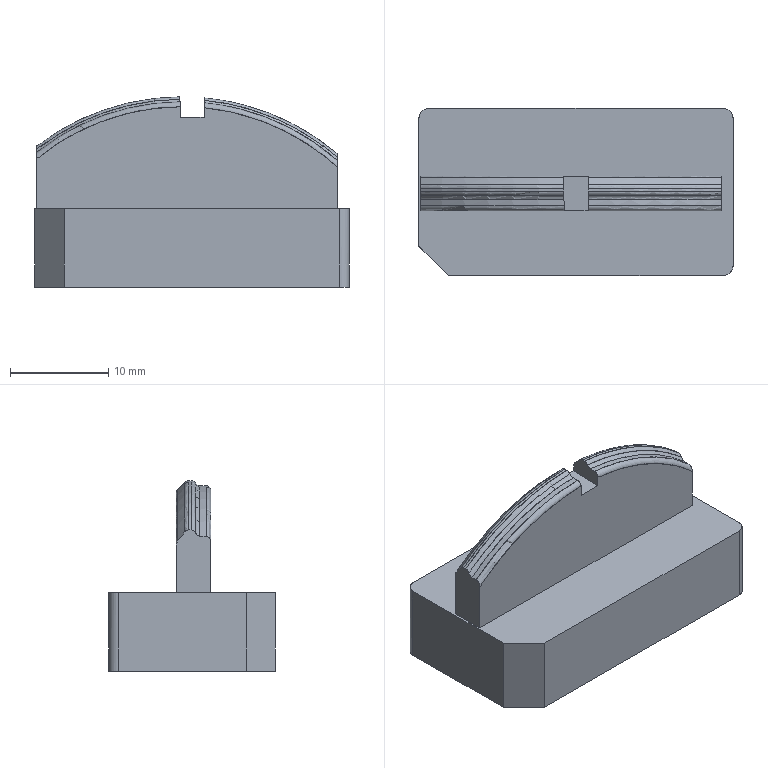NC program | PowerMill | posted with a generic post | part box 32 x 17 x 19.383 mm
Lines 8610 to 9354 of 94163:
N8707 M6
N8708 S22000 M03
N8709 G00 G90 X0.0 Y0.0
N8710 G43 Z10.803 H22
N8711
N8712 G05 P10000 R8
N8713 X15.4268 Y-3.0703
N8714 Z-6.8835
N8715 G01 Z-8.0835 F1200.0
N8716 X15.4156 Y-3.0814 Z-8.097 F2000.0
N8717 X15.3964 Y-3.1007 Z-8.1231
N8718 X15.376 Y-3.121 Z-8.1542
N8719 X15.3523 Y-3.1447 Z-8.1945
N8720 X15.3274 Y-3.1696 Z-8.242
N8721 X15.3089 Y-3.1881 Z-8.2813
N8722 X15.295 Y-3.2021 Z-8.3142
N8723 X15.2826 Y-3.2144 Z-8.3478
N8724 X15.2414 Y-3.2443 Z-8.4199
N8725 X15.199 Y-3.2705 Z-8.4928
N8726 X15.1554 Y-3.2929 Z-8.5663
N8727 X15.1411 Y-3.2994 Z-8.5902
N8728 X15.1525 Y-3.288 Z-8.5245
N8729 X15.1666 Y-3.2739 Z-8.4598
N8730 X15.1833 Y-3.2571 Z-8.3965
N8731 X15.2025 Y-3.2379 Z-8.3352
N8732 X15.224 Y-3.2164 Z-8.2762
N8733 X15.2477 Y-3.1928 Z-8.22
N8734 X15.2732 Y-3.1672 Z-8.1668
N8735 X15.3005 Y-3.14 Z-8.117
N8736 X15.3293 Y-3.1111 Z-8.0706
N8737 X15.3595 Y-3.0809 Z-8.0279
N8738 X15.3909 Y-3.0495 Z-7.989
N8739 X15.4234 Y-3.0171 Z-7.9539
N8740 X15.4567 Y-2.9837 Z-7.9227
N8741 X15.4909 Y-2.9496 Z-7.8955
N8742 X15.5257 Y-2.9148 Z-7.8721
N8743 X15.546 Y-2.8945 Z-7.8605
N8744 X15.61 Y-2.7738 Z-7.744
N8745 X15.5875 Y-2.7964 Z-7.7488
N8746 X15.572 Y-2.8119 Z-7.7542
N8747 X15.5342 Y-2.8497 Z-7.7703
N8748 X15.4967 Y-2.8871 Z-7.7904
N8749 X15.4598 Y-2.9241 Z-7.8144
N8750 X15.4234 Y-2.9604 Z-7.8424
N8751 X15.3878 Y-2.996 Z-7.8743
N8752 X15.3531 Y-3.0307 Z-7.9101
N8753 X15.3195 Y-3.0644 Z-7.9497
N8754 X15.2879 Y-3.0959 Z-7.9919
N8755 X15.2579 Y-3.126 Z-8.0376
N8756 X15.2291 Y-3.1548 Z-8.087
N8757 X15.2018 Y-3.1821 Z-8.1402
N8758 X15.1762 Y-3.2077 Z-8.1968
N8759 X15.1525 Y-3.2314 Z-8.2566
N8760 X15.1309 Y-3.253 Z-8.3191
N8761 X15.1116 Y-3.2723 Z-8.3838
N8762 X15.095 Y-3.2889 Z-8.45
N8763 X15.0811 Y-3.3028 Z-8.5166
N8764 X15.0702 Y-3.3137 Z-8.5828
N8765 X15.0621 Y-3.3217 Z-8.6478
N8766 X14.9924 Y-3.3349 Z-8.675
N8767 X14.9992 Y-3.3281 Z-8.608
N8768 X15.0089 Y-3.3184 Z-8.5397
N8769 X15.0217 Y-3.3056 Z-8.4697
N8770 X15.0377 Y-3.2896 Z-8.3981
N8771 X15.0557 Y-3.2716 Z-8.3289
N8772 X15.0757 Y-3.2516 Z-8.2631
N8773 X15.0976 Y-3.2297 Z-8.2007
N8774 X15.1214 Y-3.2059 Z-8.1417
N8775 X15.147 Y-3.1803 Z-8.0858
N8776 X15.1745 Y-3.1528 Z-8.0331
N8777 X15.2038 Y-3.1235 Z-7.9835
N8778 X15.2349 Y-3.0924 Z-7.9367
N8779 X15.2665 Y-3.0608 Z-7.8947
N8780 X15.299 Y-3.0284 Z-7.8564
N8781 X15.3344 Y-2.9929 Z-7.8197
N8782 X15.3723 Y-2.955 Z-7.7852
N8783 X15.4115 Y-2.9158 Z-7.7544
N8784 X15.4509 Y-2.8764 Z-7.7277
N8785 X15.49 Y-2.8373 Z-7.7054
N8786 X15.5282 Y-2.7991 Z-7.6877
N8787 X15.5652 Y-2.7621 Z-7.6743
N8788 X15.6008 Y-2.7266 Z-7.6652
N8789 X15.6348 Y-2.6925 Z-7.6601
N8790 X15.6524 Y-2.6749 Z-7.659
N8791 X15.6845 Y-2.5863 Z-7.5915
N8792 X15.6827 Y-2.588 Z-7.5913
N8793 X15.6486 Y-2.6222 Z-7.59
N8794 X15.6126 Y-2.6582 Z-7.5924
N8795 X15.5749 Y-2.6959 Z-7.5989
N8796 X15.5355 Y-2.7352 Z-7.6094
N8797 X15.4947 Y-2.776 Z-7.6242
N8798 X15.4528 Y-2.818 Z-7.6435
N8799 X15.4102 Y-2.8606 Z-7.6672
N8800 X15.3676 Y-2.9031 Z-7.6951
N8801 X15.326 Y-2.9447 Z-7.7268
N8802 X15.2868 Y-2.984 Z-7.761
N8803 X15.2505 Y-3.0202 Z-7.7969
N8804 X15.2176 Y-3.0532 Z-7.8339
N8805 X15.1882 Y-3.0826 Z-7.8714
N8806 X15.1612 Y-3.1095 Z-7.9101
N8807 X15.1314 Y-3.1394 Z-7.9582
N8808 X15.1032 Y-3.1676 Z-8.0097
N8809 X15.0766 Y-3.1941 Z-8.0646
N8810 X15.0517 Y-3.219 Z-8.123
N8811 X15.0287 Y-3.242 Z-8.1847
N8812 X15.0076 Y-3.2632 Z-8.2499
N8813 X14.9884 Y-3.2823 Z-8.3183
N8814 X14.9714 Y-3.2994 Z-8.3899
N8815 X14.9566 Y-3.3141 Z-8.4643
N8816 X14.9442 Y-3.3265 Z-8.5414
N8817 X14.9343 Y-3.3364 Z-8.6204
N8818 X14.927 Y-3.3437 Z-8.7008
N8819 X14.8662 Y-3.348 Z-8.6975
N8820 X14.8731 Y-3.341 Z-8.6103
N8821 X14.8824 Y-3.3317 Z-8.527
N8822 X14.894 Y-3.3201 Z-8.4474
N8823 X14.9079 Y-3.3063 Z-8.3713
N8824 X14.9239 Y-3.2903 Z-8.2984
N8825 X14.9417 Y-3.2725 Z-8.2303
N8826 X14.9615 Y-3.2526 Z-8.1649
N8827 X14.9835 Y-3.2307 Z-8.1026
N8828 X15.0074 Y-3.2068 Z-8.0433
N8829 X15.0333 Y-3.1809 Z-7.987
N8830 X15.0611 Y-3.1531 Z-7.9337
N8831 X15.0908 Y-3.1234 Z-7.8834
N8832 X15.1224 Y-3.0918 Z-7.836
N8833 X15.1558 Y-3.0584 Z-7.7916
N8834 X15.189 Y-3.0251 Z-7.7526
N8835 X15.2246 Y-2.9896 Z-7.716
N8836 X15.2625 Y-2.9517 Z-7.6819
N8837 X15.3026 Y-2.9116 Z-7.6506
N8838 X15.3448 Y-2.8694 Z-7.622
N8839 X15.3732 Y-2.841 Z-7.6052
N8840 X15.4021 Y-2.8121 Z-7.5901
N8841 X15.4316 Y-2.7826 Z-7.5765
N8842 X15.466 Y-2.7482 Z-7.5628
N8843 X15.506 Y-2.7082 Z-7.5494
N8844 X15.5505 Y-2.6637 Z-7.5379
N8845 X15.5927 Y-2.6215 Z-7.5306
N8846 X15.6313 Y-2.5828 Z-7.5274
N8847 X15.6664 Y-2.5478 Z-7.5279
N8848 X15.6982 Y-2.516 Z-7.5318
N8849 X15.7135 Y-2.5007 Z-7.535
N8850 X15.7387 Y-2.4189 Z-7.4879
N8851 X15.7303 Y-2.4273 Z-7.4851
N8852 X15.7013 Y-2.4563 Z-7.4777
N8853 X15.6691 Y-2.4885 Z-7.4728
N8854 X15.6332 Y-2.5244 Z-7.4708
N8855 X15.5932 Y-2.5644 Z-7.472
N8856 X15.5488 Y-2.6088 Z-7.4769
N8857 X15.5002 Y-2.6574 Z-7.486
N8858 X15.4505 Y-2.7071 Z-7.499
N8859 X15.406 Y-2.7516 Z-7.514
N8860 X15.3672 Y-2.7904 Z-7.5297
N8861 X15.3336 Y-2.824 Z-7.5457
N8862 X15.3047 Y-2.8529 Z-7.5615
N8863 X15.2705 Y-2.8871 Z-7.5831
N8864 X15.2299 Y-2.9277 Z-7.6124
N8865 X15.1908 Y-2.9668 Z-7.645
N8866 X15.1534 Y-3.0042 Z-7.6808
N8867 X15.1176 Y-3.04 Z-7.7197
N8868 X15.0835 Y-3.0741 Z-7.7618
N8869 X15.0511 Y-3.1065 Z-7.807
N8870 X15.0205 Y-3.1371 Z-7.8554
N8871 X14.9917 Y-3.1659 Z-7.9068
N8872 X14.9648 Y-3.1928 Z-7.9613
N8873 X14.9399 Y-3.2177 Z-8.0189
N8874 X14.9169 Y-3.2407 Z-8.0794
N8875 X14.8959 Y-3.2617 Z-8.1429
N8876 X14.877 Y-3.2806 Z-8.2092
N8877 X14.86 Y-3.2976 Z-8.2794
N8878 X14.845 Y-3.3126 Z-8.3533
N8879 X14.8321 Y-3.3255 Z-8.431
N8880 X14.8215 Y-3.3361 Z-8.5126
N8881 X14.8132 Y-3.3444 Z-8.598
N8882 X14.8073 Y-3.3503 Z-8.687
N8883 X14.7489 Y-3.3521 Z-8.6765
N8884 X14.7535 Y-3.3475 Z-8.5876
N8885 X14.7607 Y-3.3404 Z-8.5016
N8886 X14.7702 Y-3.3308 Z-8.4187
N8887 X14.7821 Y-3.3189 Z-8.3393
N8888 X14.7963 Y-3.3047 Z-8.2633
N8889 X14.8126 Y-3.2885 Z-8.1908
N8890 X14.8309 Y-3.2701 Z-8.1219
N8891 X14.8512 Y-3.2498 Z-8.0563
N8892 X14.8734 Y-3.2276 Z-7.9942
N8893 X14.8975 Y-3.2036 Z-7.9354
N8894 X14.9233 Y-3.1777 Z-7.88
N8895 X14.951 Y-3.1501 Z-7.8278
N8896 X14.9803 Y-3.1207 Z-7.7788
N8897 X15.0113 Y-3.0897 Z-7.7329
N8898 X15.044 Y-3.057 Z-7.6902
N8899 X15.0787 Y-3.0223 Z-7.6502
N8900 X15.1155 Y-2.9856 Z-7.6128
N8901 X15.154 Y-2.947 Z-7.5786
N8902 X15.1944 Y-2.9067 Z-7.5474
N8903 X15.2364 Y-2.8646 Z-7.5194
N8904 X15.2801 Y-2.8209 Z-7.4947
N8905 X15.3253 Y-2.7757 Z-7.4735
N8906 X15.3718 Y-2.7292 Z-7.4558
N8907 X15.4196 Y-2.6815 Z-7.4418
N8908 X15.4683 Y-2.6327 Z-7.4314
N8909 X15.5236 Y-2.5775 Z-7.4229
N8910 X15.5727 Y-2.5284 Z-7.4186
N8911 X15.6175 Y-2.4836 Z-7.4182
N8912 X15.659 Y-2.4421 Z-7.4214
N8913 X15.6978 Y-2.4032 Z-7.428
N8914 X15.7345 Y-2.3666 Z-7.4379
N8915 X15.7593 Y-2.3418 Z-7.447
N8916 X15.7805 Y-2.264 Z-7.4113
N8917 X15.7689 Y-2.2756 Z-7.4063
N8918 X15.7299 Y-2.3145 Z-7.3921
N8919 X15.6887 Y-2.3558 Z-7.3811
N8920 X15.645 Y-2.3995 Z-7.3733
N8921 X15.5982 Y-2.4462 Z-7.3689
N8922 X15.5478 Y-2.4967 Z-7.3681
N8923 X15.4927 Y-2.5518 Z-7.3709
N8924 X15.4411 Y-2.6034 Z-7.3765
N8925 X15.3906 Y-2.6538 Z-7.3853
N8926 X15.3415 Y-2.703 Z-7.3978
N8927 X15.2937 Y-2.7507 Z-7.4139
N8928 X15.2476 Y-2.7969 Z-7.4334
N8929 X15.203 Y-2.8414 Z-7.4564
N8930 X15.1603 Y-2.8842 Z-7.4826
N8931 X15.1193 Y-2.9251 Z-7.5119
N8932 X15.0802 Y-2.9642 Z-7.5443
N8933 X15.0429 Y-3.0016 Z-7.5797
N8934 X15.0073 Y-3.0371 Z-7.618
N8935 X14.9735 Y-3.071 Z-7.6592
N8936 X14.9413 Y-3.1032 Z-7.7034
N8937 X14.9109 Y-3.1336 Z-7.7507
N8938 X14.8822 Y-3.1623 Z-7.801
N8939 X14.8552 Y-3.1892 Z-7.8545
N8940 X14.8301 Y-3.2143 Z-7.9111
N8941 X14.8069 Y-3.2376 Z-7.971
N8942 X14.7855 Y-3.259 Z-8.0342
N8943 X14.7661 Y-3.2784 Z-8.1008
N8944 X14.7487 Y-3.2958 Z-8.1708
N8945 X14.7334 Y-3.3111 Z-8.2444
N8946 X14.7203 Y-3.3242 Z-8.3214
N8947 X14.7094 Y-3.3351 Z-8.402
N8948 X14.7008 Y-3.3436 Z-8.4862
N8949 X14.6947 Y-3.3497 Z-8.5738
N8950 X14.6912 Y-3.3533 Z-8.6645
N8951 X14.6337 Y-3.3542 Z-8.6512
N8952 X14.6363 Y-3.3516 Z-8.5591
N8953 X14.6415 Y-3.3464 Z-8.4701
N8954 X14.6492 Y-3.3387 Z-8.3845
N8955 X14.6593 Y-3.3286 Z-8.3024
N8956 X14.6716 Y-3.3163 Z-8.2238
N8957 X14.6862 Y-3.3017 Z-8.1488
N8958 X14.7028 Y-3.2851 Z-8.0774
N8959 X14.7215 Y-3.2664 Z-8.0094
N8960 X14.7422 Y-3.2457 Z-7.9448
N8961 X14.7648 Y-3.2231 Z-7.8836
N8962 X14.7892 Y-3.1987 Z-7.8257
N8963 X14.8155 Y-3.1724 Z-7.771
N8964 X14.8435 Y-3.1444 Z-7.7196
N8965 X14.8733 Y-3.1146 Z-7.6712
N8966 X14.9048 Y-3.0831 Z-7.626
N8967 X14.938 Y-3.0499 Z-7.5838
N8968 X14.9728 Y-3.0151 Z-7.5446
N8969 X15.0092 Y-2.9787 Z-7.5085
N8970 X15.0469 Y-2.941 Z-7.4755
N8971 X15.0864 Y-2.9015 Z-7.4454
N8972 X15.1278 Y-2.8601 Z-7.4183
N8973 X15.1714 Y-2.8165 Z-7.3941
N8974 X15.2175 Y-2.7704 Z-7.3727
N8975 X15.2661 Y-2.7218 Z-7.3542
N8976 X15.2963 Y-2.6916 Z-7.3445
N8977 X15.3272 Y-2.6607 Z-7.3366
N8978 X15.3628 Y-2.6251 Z-7.3297
N8979 X15.4038 Y-2.5841 Z-7.324
N8980 X15.451 Y-2.5369 Z-7.32
N8981 X15.5051 Y-2.4828 Z-7.3186
N8982 X15.5629 Y-2.425 Z-7.3207
N8983 X15.6147 Y-2.3732 Z-7.326
N8984 X15.6602 Y-2.3277 Z-7.3336
N8985 X15.7 Y-2.2879 Z-7.343
N8986 X15.7349 Y-2.253 Z-7.3539
N8987 X15.7656 Y-2.2223 Z-7.3661
N8988 X15.7946 Y-2.1933 Z-7.3808
N8989 X15.797 Y-2.1909 Z-7.3822
N8990 X15.8099 Y-2.1214 Z-7.3564
N8991 X15.7858 Y-2.1455 Z-7.3418
N8992 X15.7525 Y-2.1789 Z-7.3253
N8993 X15.7148 Y-2.2166 Z-7.3105
N8994 X15.6718 Y-2.2595 Z-7.2976
N8995 X15.6227 Y-2.3086 Z-7.2866
N8996 X15.568 Y-2.3634 Z-7.2778
N8997 X15.5206 Y-2.4108 Z-7.2724
N8998 X15.4638 Y-2.4675 Z-7.2688
N8999 X15.4086 Y-2.5228 Z-7.2692
N9000 X15.3547 Y-2.5766 Z-7.2734
N9001 X15.3023 Y-2.629 Z-7.2814
N9002 X15.2513 Y-2.68 Z-7.2931
N9003 X15.2017 Y-2.7297 Z-7.3084
N9004 X15.1534 Y-2.778 Z-7.3273
N9005 X15.1095 Y-2.8218 Z-7.348
N9006 X15.0666 Y-2.8647 Z-7.3723
N9007 X15.0249 Y-2.9064 Z-7.4001
N9008 X14.9846 Y-2.9467 Z-7.4315
N9009 X14.9458 Y-2.9855 Z-7.4662
N9010 X14.9087 Y-3.0227 Z-7.5042
N9011 X14.8732 Y-3.0581 Z-7.5453
N9012 X14.8396 Y-3.0917 Z-7.5895
N9013 X14.8079 Y-3.1234 Z-7.6365
N9014 X14.7783 Y-3.153 Z-7.6863
N9015 X14.7507 Y-3.1806 Z-7.7388
N9016 X14.725 Y-3.2063 Z-7.7942
N9017 X14.7012 Y-3.2301 Z-7.8529
N9018 X14.6793 Y-3.2521 Z-7.9147
N9019 X14.6592 Y-3.2721 Z-7.98
N9020 X14.6412 Y-3.2901 Z-8.0487
N9021 X14.6252 Y-3.3061 Z-8.121
N9022 X14.6113 Y-3.32 Z-8.1969
N9023 X14.5995 Y-3.3318 Z-8.2766
N9024 X14.5901 Y-3.3412 Z-8.3602
N9025 X14.5831 Y-3.3482 Z-8.4467
N9026 X14.5786 Y-3.3527 Z-8.5365
N9027 X14.5768 Y-3.3545 Z-8.6297
N9028 Z-8.638
N9029 X14.5202 Y-3.3546 Z-8.6211
N9030 Z-8.5883
N9031 X14.5218 Y-3.3529 Z-8.4943
N9032 X14.5261 Y-3.3487 Z-8.4039
N9033 X14.5329 Y-3.3419 Z-8.317
N9034 X14.542 Y-3.3327 Z-8.2339
N9035 X14.5535 Y-3.3213 Z-8.1544
N9036 X14.5672 Y-3.3076 Z-8.0786
N9037 X14.583 Y-3.2917 Z-8.0062
N9038 X14.6009 Y-3.2738 Z-7.9373
N9039 X14.6209 Y-3.2539 Z-7.8717
N9040 X14.6428 Y-3.232 Z-7.8094
N9041 X14.6666 Y-3.2082 Z-7.7503
N9042 X14.6923 Y-3.1825 Z-7.6943
N9043 X14.7198 Y-3.1549 Z-7.6415
N9044 X14.7492 Y-3.1256 Z-7.5917
N9045 X14.7803 Y-3.0944 Z-7.5449
N9046 X14.8132 Y-3.0615 Z-7.501
N9047 X14.8477 Y-3.027 Z-7.4603
N9048 X14.8838 Y-2.9909 Z-7.4228
N9049 X14.9216 Y-2.9531 Z-7.3885
N9050 X14.9613 Y-2.9134 Z-7.357
N9051 X15.003 Y-2.8717 Z-7.3286
N9052 X15.0467 Y-2.8281 Z-7.3031
N9053 X15.0923 Y-2.7825 Z-7.2809
N9054 X15.1399 Y-2.7348 Z-7.2618
N9055 X15.1895 Y-2.6853 Z-7.246
N9056 X15.2411 Y-2.6337 Z-7.2337
N9057 X15.2946 Y-2.5802 Z-7.2248
N9058 X15.35 Y-2.5248 Z-7.2197
N9059 X15.3784 Y-2.4963 Z-7.2186
N9060 X15.4073 Y-2.4675 Z-7.2188
N9061 X15.441 Y-2.4337 Z-7.2205
N9062 X15.4806 Y-2.3941 Z-7.2241
N9063 X15.5278 Y-2.3469 Z-7.2304
N9064 X15.5849 Y-2.2899 Z-7.2408
N9065 X15.6404 Y-2.2344 Z-7.254
N9066 X15.6863 Y-2.1885 Z-7.2678
N9067 X15.725 Y-2.1498 Z-7.2817
N9068 X15.7579 Y-2.1168 Z-7.296
N9069 X15.7861 Y-2.0887 Z-7.3104
N9070 X15.812 Y-2.0628 Z-7.3264
N9071 X15.8212 Y-2.0536 Z-7.3329
N9072 X15.8305 Y-1.9877 Z-7.3116
N9073 X15.8244 Y-1.9938 Z-7.307
N9074 X15.7966 Y-2.0216 Z-7.2886
N9075 X15.7675 Y-2.0507 Z-7.2722
N9076 X15.7335 Y-2.0847 Z-7.2558
N9077 X15.6936 Y-2.1246 Z-7.2392
N9078 X15.6464 Y-2.1718 Z-7.2226
N9079 X15.5896 Y-2.2286 Z-7.2058
N9080 X15.5304 Y-2.2878 Z-7.1917
N9081 X15.4811 Y-2.3371 Z-7.1824
N9082 X15.4395 Y-2.3787 Z-7.1763
N9083 X15.4039 Y-2.4143 Z-7.1725
N9084 X15.3731 Y-2.4451 Z-7.1704
N9085 X15.3423 Y-2.4759 Z-7.1698
N9086 X15.2844 Y-2.5338 Z-7.1718
N9087 X15.2294 Y-2.5888 Z-7.1773
N9088 X15.1769 Y-2.6413 Z-7.1864
N9089 X15.1266 Y-2.6915 Z-7.1988
N9090 X15.0785 Y-2.7397 Z-7.2146
N9091 X15.0322 Y-2.786 Z-7.2337
N9092 X14.9876 Y-2.8306 Z-7.2562
N9093 X14.9446 Y-2.8736 Z-7.2819
N9094 X14.9031 Y-2.9151 Z-7.3108
N9095 X14.8638 Y-2.9544 Z-7.3423
N9096 X14.826 Y-2.9922 Z-7.3768
N9097 X14.7899 Y-3.0283 Z-7.4142
N9098 X14.7555 Y-3.0627 Z-7.4546
N9099 X14.7228 Y-3.0954 Z-7.498
N9100 X14.6918 Y-3.1264 Z-7.5445
N9101 X14.6626 Y-3.1556 Z-7.594
N9102 X14.6352 Y-3.183 Z-7.6467
N9103 X14.6096 Y-3.2086 Z-7.7025
N9104 X14.5858 Y-3.2324 Z-7.7616
N9105 X14.564 Y-3.2542 Z-7.8239
N9106 X14.5441 Y-3.274 Z-7.8895
N9107 X14.5263 Y-3.2919 Z-7.9586
N9108 X14.5105 Y-3.3077 Z-8.031
N9109 X14.4968 Y-3.3214 Z-8.107
N9110 X14.4853 Y-3.3329 Z-8.1866
N9111 X14.4762 Y-3.342 Z-8.2693
N9112 X14.4695 Y-3.3487 Z-8.3555
N9113 X14.4653 Y-3.3529 Z-8.4455
N9114 X14.4636 Y-3.3546 Z-8.5398
N9115 Z-8.5922
N9116 X14.407 Z-8.5633
N9117 Z-8.4931
N9118 X14.4085 Y-3.3531 Z-8.4005
N9119 X14.4126 Y-3.349 Z-8.3114
N9120 X14.4193 Y-3.3423 Z-8.2247
N9121 X14.4285 Y-3.3332 Z-8.1406
N9122 X14.4397 Y-3.3219 Z-8.0612
N9123 X14.4531 Y-3.3085 Z-7.9858
N9124 X14.4686 Y-3.293 Z-7.9142
N9125 X14.4862 Y-3.2755 Z-7.846
N9126 X14.5058 Y-3.2558 Z-7.781
N9127 X14.5275 Y-3.2341 Z-7.719
N9128 X14.5512 Y-3.2104 Z-7.6598
N9129 X14.577 Y-3.1847 Z-7.6034
N9130 X14.6049 Y-3.1567 Z-7.5492
N9131 X14.634 Y-3.1277 Z-7.4993
N9132 X14.665 Y-3.0966 Z-7.4521
N9133 X14.698 Y-3.0636 Z-7.4079
N9134 X14.7329 Y-3.0288 Z-7.3666
N9135 X14.7696 Y-2.9921 Z-7.3283
N9136 X14.808 Y-2.9536 Z-7.2932
N9137 X14.8481 Y-2.9135 Z-7.2612
N9138 X14.8899 Y-2.8717 Z-7.2326
N9139 X14.9329 Y-2.8287 Z-7.2075
N9140 X14.9796 Y-2.782 Z-7.1845
N9141 X15.0272 Y-2.7344 Z-7.1651
N9142 X15.0763 Y-2.6854 Z-7.1492
N9143 X15.1269 Y-2.6348 Z-7.1368
N9144 X15.1793 Y-2.5823 Z-7.128
N9145 X15.2337 Y-2.5279 Z-7.1228
N9146 X15.2905 Y-2.4711 Z-7.1212
N9147 X15.343 Y-2.4186 Z-7.123
N9148 X15.377 Y-2.3846 Z-7.126
N9149 X15.4115 Y-2.3501 Z-7.1306
N9150 X15.4514 Y-2.3103 Z-7.1376
N9151 X15.4979 Y-2.2637 Z-7.1476
N9152 X15.5531 Y-2.2085 Z-7.1619
N9153 X15.6176 Y-2.1441 Z-7.182
N9154 X15.6719 Y-2.0897 Z-7.2022
N9155 X15.7176 Y-2.0441 Z-7.2217
N9156 X15.7564 Y-2.0052 Z-7.2408
N9157 X15.7897 Y-1.9719 Z-7.2595
N9158 X15.8206 Y-1.9411 Z-7.2794
N9159 X15.8389 Y-1.9228 Z-7.2929
N9160 X15.8444 Y-1.8606 Z-7.2786
N9161 X15.8234 Y-1.8817 Z-7.2611
N9162 X15.7936 Y-1.9115 Z-7.2398
N9163 X15.7582 Y-1.9469 Z-7.2182
N9164 X15.7154 Y-1.9897 Z-7.1958
N9165 X15.6628 Y-2.0423 Z-7.1721
N9166 X15.6171 Y-2.0879 Z-7.1538
N9167 X15.5801 Y-2.1249 Z-7.14
N9168 X15.5453 Y-2.1597 Z-7.1277
N9169 X15.482 Y-2.2231 Z-7.1084
N9170 X15.4203 Y-2.2848 Z-7.0934
N9171 X15.3599 Y-2.3451 Z-7.0826
N9172 X15.3008 Y-2.4042 Z-7.0759
N9173 X15.2428 Y-2.4623 Z-7.0732
N9174 X15.185 Y-2.52 Z-7.0744
N9175 X15.1297 Y-2.5754 Z-7.0794
N9176 X15.0762 Y-2.6288 Z-7.0879
N9177 X15.0248 Y-2.6802 Z-7.0999
N9178 X14.9754 Y-2.7296 Z-7.1153
N9179 X14.928 Y-2.7771 Z-7.1341
N9180 X14.8824 Y-2.8227 Z-7.1561
N9181 X14.8386 Y-2.8664 Z-7.1814
N9182 X14.7967 Y-2.9084 Z-7.2098
N9183 X14.7565 Y-2.9485 Z-7.2413
N9184 X14.7181 Y-2.9869 Z-7.2759
N9185 X14.6815 Y-3.0236 Z-7.3135
N9186 X14.6465 Y-3.0585 Z-7.3541
N9187 X14.6136 Y-3.0915 Z-7.3974
N9188 X14.5822 Y-3.1229 Z-7.4438
N9189 X14.5528 Y-3.1523 Z-7.4929
N9190 X14.5252 Y-3.1799 Z-7.5452
N9191 X14.4993 Y-3.2057 Z-7.6007
N9192 X14.4753 Y-3.2297 Z-7.6593
N9193 X14.4532 Y-3.2518 Z-7.7213
N9194 X14.4331 Y-3.272 Z-7.7865
N9195 X14.4149 Y-3.2902 Z-7.8552
N9196 X14.3988 Y-3.3063 Z-7.9273
N9197 X14.3848 Y-3.3202 Z-8.0028
N9198 X14.3731 Y-3.3319 Z-8.0818
N9199 X14.3637 Y-3.3413 Z-8.1643
N9200 X14.3568 Y-3.3483 Z-8.25
N9201 X14.3524 Y-3.3527 Z-8.3387
N9202 X14.3505 Y-3.3545 Z-8.4322
N9203 Z-8.5344
N9204 X14.2939 Y-3.3546 Z-8.489
N9205 Z-8.3864
N9206 X14.2956 Y-3.3529 Z-8.2949
N9207 X14.3 Y-3.3485 Z-8.2059
N9208 X14.3069 Y-3.3415 Z-8.1195
N9209 X14.3165 Y-3.332 Z-8.0356
N9210 X14.327 Y-3.3215 Z-7.9629
N9211 X14.3405 Y-3.308 Z-7.8881
N9212 X14.3562 Y-3.2923 Z-7.8164
N9213 X14.374 Y-3.2744 Z-7.7476
N9214 X14.394 Y-3.2545 Z-7.682
N9215 X14.416 Y-3.2325 Z-7.6195
N9216 X14.44 Y-3.2085 Z-7.5601
N9217 X14.4658 Y-3.1826 Z-7.5039
N9218 X14.4936 Y-3.1549 Z-7.4508
N9219 X14.5231 Y-3.1254 Z-7.4008
N9220 X14.5543 Y-3.0942 Z-7.3539
N9221 X14.5873 Y-3.0612 Z-7.3102
N9222 X14.6219 Y-3.0266 Z-7.2695
N9223 X14.6582 Y-2.9903 Z-7.232
N9224 X14.6962 Y-2.9523 Z-7.1974
N9225 X14.7366 Y-2.9119 Z-7.1653
N9226 X14.7788 Y-2.8697 Z-7.1363
N9227 X14.8228 Y-2.8257 Z-7.1105
N9228 X14.8685 Y-2.78 Z-7.088
N9229 X14.9158 Y-2.7327 Z-7.0689
N9230 X14.9645 Y-2.684 Z-7.0534
N9231 X15.0141 Y-2.6344 Z-7.0414
N9232 X15.0675 Y-2.581 Z-7.0322
N9233 X15.122 Y-2.5265 Z-7.0267
N9234 X15.178 Y-2.4705 Z-7.0249
N9235 X15.2358 Y-2.4127 Z-7.027
N9236 X15.2957 Y-2.3527 Z-7.0332
N9237 X15.3582 Y-2.2903 Z-7.0434
N9238 X15.3876 Y-2.2609 Z-7.0494
N9239 X15.4158 Y-2.2327 Z-7.0562
N9240 X15.4442 Y-2.2043 Z-7.0641
N9241 X15.4774 Y-2.1711 Z-7.0744
N9242 X15.5167 Y-2.1318 Z-7.0878
N9243 X15.5642 Y-2.0843 Z-7.1056
N9244 X15.6245 Y-2.024 Z-7.1306
N9245 X15.6799 Y-1.9686 Z-7.1564
N9246 X15.7238 Y-1.9247 Z-7.1791
N9247 X15.76 Y-1.8885 Z-7.1998
N9248 X15.7905 Y-1.858 Z-7.2191
N9249 X15.8162 Y-1.8323 Z-7.2373
N9250 X15.8408 Y-1.8077 Z-7.2572
N9251 X15.8491 Y-1.7994 Z-7.2648
N9252 X15.855 Y-1.737 Z-7.2543
N9253 X15.8285 Y-1.7634 Z-7.2313
N9254 X15.7978 Y-1.7942 Z-7.2078
N9255 X15.7642 Y-1.8277 Z-7.1848
N9256 X15.7251 Y-1.8668 Z-7.1606
N9257 X15.6791 Y-1.9128 Z-7.1348
N9258 X15.6241 Y-1.9678 Z-7.1069
N9259 X15.5572 Y-2.0348 Z-7.0766
N9260 X15.4966 Y-2.0953 Z-7.0522
N9261 X15.446 Y-2.146 Z-7.034
N9262 X15.4026 Y-2.1893 Z-7.02
N9263 X15.3651 Y-2.2269 Z-7.0092
N9264 X15.3304 Y-2.2615 Z-7.0007
N9265 X15.2956 Y-2.2964 Z-6.9937
N9266 X15.2388 Y-2.3532 Z-6.985
N9267 X15.1802 Y-2.4117 Z-6.9791
N9268 X15.123 Y-2.4689 Z-6.9769
N9269 X15.069 Y-2.5229 Z-6.9785
N9270 X15.0168 Y-2.5751 Z-6.9836
N9271 X14.9647 Y-2.6272 Z-6.9921
N9272 X14.9164 Y-2.6755 Z-7.0034
N9273 X14.8669 Y-2.725 Z-7.0188
N9274 X14.8191 Y-2.7729 Z-7.0376
N9275 X14.7729 Y-2.819 Z-7.0598
N9276 X14.7286 Y-2.8633 Z-7.0853
N9277 X14.6862 Y-2.9057 Z-7.1138
N9278 X14.6457 Y-2.9462 Z-7.1454
N9279 X14.6072 Y-2.9848 Z-7.1799
N9280 X14.5705 Y-3.0214 Z-7.2173
N9281 X14.5355 Y-3.0564 Z-7.2577
N9282 X14.5023 Y-3.0896 Z-7.301
N9283 X14.4708 Y-3.1211 Z-7.3472
N9284 X14.4412 Y-3.1508 Z-7.3965
N9285 X14.4133 Y-3.1786 Z-7.4487
N9286 X14.3873 Y-3.2047 Z-7.504
N9287 X14.3631 Y-3.2288 Z-7.5625
N9288 X14.3409 Y-3.251 Z-7.6241
N9289 X14.3207 Y-3.2713 Z-7.689
N9290 X14.3024 Y-3.2895 Z-7.7572
N9291 X14.2863 Y-3.3056 Z-7.8287
N9292 X14.2723 Y-3.3196 Z-7.9037
N9293 X14.2605 Y-3.3314 Z-7.9822
N9294 X14.251 Y-3.3409 Z-8.0643
N9295 X14.2439 Y-3.348 Z-8.1499
N9296 X14.2393 Y-3.3526 Z-8.239
N9297 X14.2374 Y-3.3545 Z-8.3316
N9298 Z-8.4414
N9299 X14.1808 Z-8.3939
N9300 Z-8.2834
N9301 X14.1828 Y-3.3525 Z-8.1903
N9302 X14.1875 Y-3.3479 Z-8.101
N9303 X14.1945 Y-3.3408 Z-8.0157
N9304 X14.204 Y-3.3314 Z-7.934
N9305 X14.2157 Y-3.3196 Z-7.8559
N9306 X14.2297 Y-3.3056 Z-7.7814
N9307 X14.2459 Y-3.2895 Z-7.7102
N9308 X14.2641 Y-3.2713 Z-7.6423
N9309 X14.2844 Y-3.251 Z-7.5775
N9310 X14.3067 Y-3.2286 Z-7.5158
N9311 X14.331 Y-3.2043 Z-7.4571
N9312 X14.3573 Y-3.1781 Z-7.4013
N9313 X14.3849 Y-3.1504 Z-7.3494
N9314 X14.4146 Y-3.1208 Z-7.3
N9315 X14.4462 Y-3.0891 Z-7.2535
N9316 X14.4798 Y-3.0556 Z-7.2098
N9317 X14.5152 Y-3.0202 Z-7.169
N9318 X14.5525 Y-2.9829 Z-7.1313
N9319 X14.5916 Y-2.9437 Z-7.0965
N9320 X14.6325 Y-2.9028 Z-7.0649
N9321 X14.6751 Y-2.8602 Z-7.0366
N9322 X14.7194 Y-2.8159 Z-7.0114
N9323 X14.7654 Y-2.77 Z-6.9897
N9324 X14.8125 Y-2.7228 Z-6.9713
N9325 X14.8631 Y-2.6723 Z-6.9557
N9326 X14.9151 Y-2.6202 Z-6.9436
N9327 X14.9688 Y-2.5666 Z-6.9352
N9328 X15.0241 Y-2.5113 Z-6.9304
N9329 X15.081 Y-2.4543 Z-6.9295
N9330 X15.1397 Y-2.3957 Z-6.9325
N9331 X15.2 Y-2.3353 Z-6.9395
N9332 X15.2621 Y-2.2732 Z-6.9507
N9333 X15.326 Y-2.2094 Z-6.9661
N9334 X15.3915 Y-2.1439 Z-6.9859
N9335 X15.4585 Y-2.0769 Z-7.0102
N9336 X15.521 Y-2.0143 Z-7.0364
N9337 X15.5469 Y-1.9885 Z-7.0481
N9338 X15.5758 Y-1.9596 Z-7.062
N9339 X15.6107 Y-1.9247 Z-7.0795
N9340 X15.6544 Y-1.881 Z-7.1027
N9341 X15.7121 Y-1.8232 Z-7.136
N9342 X15.7543 Y-1.7811 Z-7.1626
N9343 X15.7876 Y-1.7477 Z-7.1857
N9344 X15.8149 Y-1.7204 Z-7.2065
N9345 X15.838 Y-1.6973 Z-7.2262
N9346 X15.8596 Y-1.6758 Z-7.2472
N9347 X15.8628 Y-1.616 Z-7.2413
N9348 X15.8473 Y-1.6315 Z-7.2255
N9349 X15.8147 Y-1.6641 Z-7.1958
N9350 X15.7771 Y-1.7017 Z-7.166
N9351 X15.7321 Y-1.7467 Z-7.1346
N9352 X15.6729 Y-1.8059 Z-7.0969
N9353 X15.6171 Y-1.8617 Z-7.0638
N9354 X15.5601 Y-1.9187 Z-7.033
N9355 X15.4936 Y-1.9852 Z-7.0004
N9356 X15.424 Y-2.0548 Z-6.9701
N9357 X15.362 Y-2.1168 Z-6.9464
N9358 X15.3026 Y-2.1762 Z-6.9268
N9359 X15.2534 Y-2.2254 Z-6.9133
N9360 X15.1898 Y-2.289 Z-6.8994
N9361 X15.1275 Y-2.3513 Z-6.8895
N9362 X15.067 Y-2.4118 Z-6.8838
N9363 X15.0082 Y-2.4706 Z-6.8821
N9364 X14.9514 Y-2.5274 Z-6.8842
N9365 X14.8964 Y-2.5823 Z-6.8901
N9366 X14.8434 Y-2.6354 Z-6.8996
N9367 X14.7923 Y-2.6865 Z-6.9126
N9368 X14.7431 Y-2.7357 Z-6.929
N9369 X14.6957 Y-2.7831 Z-6.9488
N9370 X14.6502 Y-2.8286 Z-6.9718
N9371 X14.607 Y-2.8718 Z-6.9977
N9372 X14.5651 Y-2.9136 Z-7.0269
N9373 X14.525 Y-2.9538 Z-7.0592
N9374 X14.4865 Y-2.9923 Z-7.0945
N9375 X14.4497 Y-3.0291 Z-7.1329
N9376 X14.4146 Y-3.0641 Z-7.1744
N9377 X14.3814 Y-3.0974 Z-7.2189
N9378 X14.35 Y-3.1288 Z-7.2665
N9379 X14.3204 Y-3.1584 Z-7.3171
N9380 X14.2927 Y-3.186 Z-7.3706
N9381 X14.2671 Y-3.2117 Z-7.4271
N9382 X14.2434 Y-3.2354 Z-7.4866
N9383 X14.2217 Y-3.2571 Z-7.5489
N9384 X14.2021 Y-3.2766 Z-7.6141
N9385 X14.1847 Y-3.2941 Z-7.6821
N9386 X14.1695 Y-3.3093 Z-7.7529
N9387 X14.1571 Y-3.3217 Z-7.822
N9388 X14.1458 Y-3.3329 Z-7.8984
N9389 X14.1369 Y-3.3419 Z-7.9774
N9390 X14.1303 Y-3.3485 Z-8.0607
N9391 X14.1261 Y-3.3527 Z-8.1481
N9392 X14.1243 Y-3.3545 Z-8.2358
N9393 X14.1242 Z-8.3465
N9394 X14.0676 Y-3.3546 Z-8.2993
N9395 Z-8.1965
N9396 X14.0694 Y-3.3528 Z-8.1034
N9397 X14.0738 Y-3.3484 Z-8.0141
N9398 X14.0807 Y-3.3415 Z-7.9286
N9399 X14.0899 Y-3.3323 Z-7.8469
N9400 X14.1015 Y-3.3207 Z-7.7688
N9401 X14.1153 Y-3.3069 Z-7.6941
N9402 X14.1312 Y-3.291 Z-7.6228
N9403 X14.1493 Y-3.2729 Z-7.5548
N9404 X14.1694 Y-3.2528 Z-7.4899
N9405 X14.1916 Y-3.2306 Z-7.4282
N9406 X14.2157 Y-3.2065 Z-7.3694
N9407 X14.2418 Y-3.1804 Z-7.3136
N9408 X14.2698 Y-3.1524 Z-7.2608
N9409 X14.3001 Y-3.1221 Z-7.2101
N9410 X14.3313 Y-3.0909 Z-7.1638
N9411 X14.3643 Y-3.0579 Z-7.1204
N9412 X14.3992 Y-3.023 Z-7.0798
N9413 X14.436 Y-2.9862 Z-7.0421
N9414 X14.4747 Y-2.9475 Z-7.0073
N9415 X14.5153 Y-2.9069 Z-6.9754
N9416 X14.5579 Y-2.8643 Z-6.9466
N9417 X14.6024 Y-2.8198 Z-6.9209
N9418 X14.6488 Y-2.7734 Z-6.8984
N9419 X14.6971 Y-2.7251 Z-6.8791
N9420 X14.7474 Y-2.6748 Z-6.8631
N9421 X14.799 Y-2.6232 Z-6.8507
N9422 X14.8524 Y-2.5698 Z-6.8419
N9423 X14.9076 Y-2.5146 Z-6.8367
N9424 X14.9646 Y-2.4576 Z-6.8353
N9425 X15.0236 Y-2.3986 Z-6.8378
N9426 X15.0847 Y-2.3376 Z-6.8443
N9427 X15.1478 Y-2.2744 Z-6.855
N9428 X15.2131 Y-2.2091 Z-6.87
N9429 X15.2806 Y-2.1416 Z-6.8894
N9430 X15.3253 Y-2.0969 Z-6.9043
N9431 X15.3588 Y-2.0634 Z-6.917
N9432 X15.3921 Y-2.0301 Z-6.9309
N9433 X15.4276 Y-1.9946 Z-6.947
N9434 X15.4688 Y-1.9534 Z-6.9668
N9435 X15.5173 Y-1.9049 Z-6.9917
N9436 X15.5766 Y-1.8456 Z-7.0244
N9437 X15.6445 Y-1.7777 Z-7.0649
N9438 X15.6979 Y-1.7243 Z-7.0995
N9439 X15.7416 Y-1.6806 Z-7.13
N9440 X15.7783 Y-1.6439 Z-7.1577
N9441 X15.8096 Y-1.6126 Z-7.1832
N9442 X15.8388 Y-1.5834 Z-7.2093
N9443 X15.8647 Y-1.5575 Z-7.2354
N9444 X15.8644 Y-1.5013 Z-7.2304
N9445 X15.8403 Y-1.5253 Z-7.2052
N9446 X15.8109 Y-1.5547 Z-7.1777
N9447 X15.7799 Y-1.5858 Z-7.1511
N9448 X15.7434 Y-1.6223 Z-7.1221
N9449 X15.7 Y-1.6656 Z-7.0901
N9450 X15.6471 Y-1.7185 Z-7.0538
N9451 X15.5795 Y-1.7861 Z-7.0107